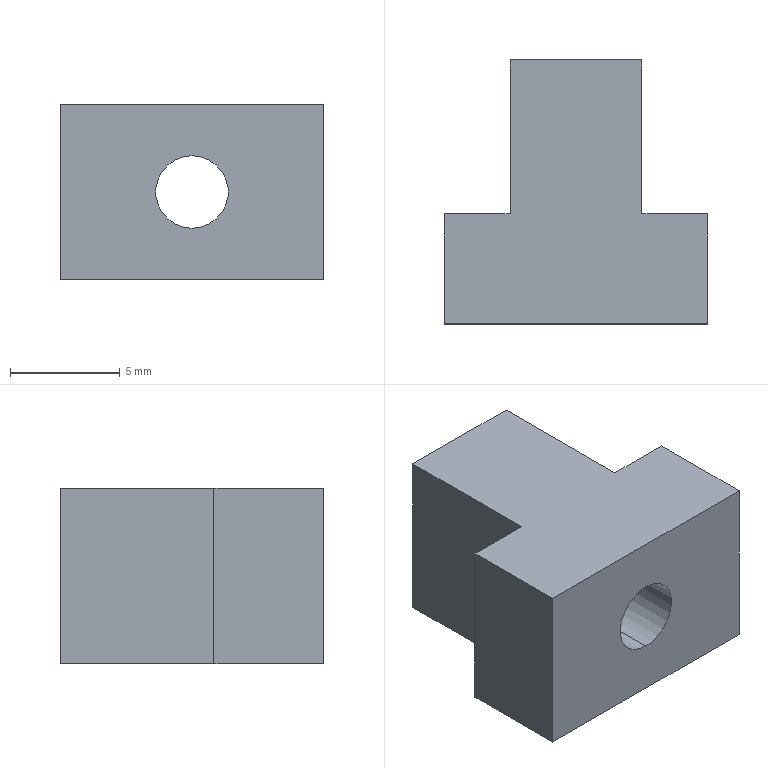Part | STEP file | Shift T-type connector | 1 solid | 12 faces | box 12 x 12 x 8 mm | volume 713.364 mm3 | plane 10 | cylinder 2 | commonest cylinder face diameters 3.3 x2
STEP:
#1=CARTESIAN_POINT('',(0.,0.,0.));
#2=DIRECTION('',(0.,0.,1.));
#3=DIRECTION('',(1.,0.,0.));
#4=AXIS2_PLACEMENT_3D('',#1,#2,#3);
#5=CARTESIAN_POINT('',(6.,0.,5.65));
#6=VERTEX_POINT('',#5);
#7=CARTESIAN_POINT('',(6.,12.,5.65));
#8=VERTEX_POINT('',#7);
#9=CARTESIAN_POINT('',(6.,12.,5.65));
#10=DIRECTION('',(0.,1.,0.));
#11=VECTOR('',#10,1.);
#12=LINE('',#9,#11);
#13=CARTESIAN_POINT('',(6.,12.,4.));
#14=DIRECTION('',(0.,1.,0.));
#15=DIRECTION('',(0.,0.,1.));
#16=AXIS2_PLACEMENT_3D('',#13,#14,#15);
#17=CYLINDRICAL_SURFACE('',#16,1.65);
#18=CARTESIAN_POINT('',(6.283,0.));
#19=DIRECTION('',(0.,1.));
#20=VECTOR('',#19,1.);
#21=LINE('',#18,#20);
#22=(GEOMETRIC_REPRESENTATION_CONTEXT(2)PARAMETRIC_REPRESENTATION_CONTEXT()REPRESENTATION_CONTEXT('',''));
#23=DEFINITIONAL_REPRESENTATION('',(#21),#22);
#24=PCURVE('',#17,#23);
#25=CARTESIAN_POINT('',(6.,12.,4.));
#26=DIRECTION('',(0.,1.,0.));
#27=DIRECTION('',(0.,0.,1.));
#28=AXIS2_PLACEMENT_3D('',#25,#26,#27);
#29=CYLINDRICAL_SURFACE('',#28,1.65);
#30=CARTESIAN_POINT('',(0.,0.));
#31=DIRECTION('',(0.,1.));
#32=VECTOR('',#31,1.);
#33=LINE('',#30,#32);
#34=(GEOMETRIC_REPRESENTATION_CONTEXT(2)PARAMETRIC_REPRESENTATION_CONTEXT()REPRESENTATION_CONTEXT('',''));
#35=DEFINITIONAL_REPRESENTATION('',(#33),#34);
#36=PCURVE('',#29,#35);
#37=SURFACE_CURVE('',#12,(#24,#36),.PCURVE_S1.);
#38=EDGE_CURVE('',#6,#8,#37,.T.);
#39=ORIENTED_EDGE('',*,*,#38,.T.);
#40=CARTESIAN_POINT('',(6.,12.,2.35));
#41=VERTEX_POINT('',#40);
#42=CARTESIAN_POINT('',(6.,12.,4.));
#43=DIRECTION('',(0.,1.,0.));
#44=DIRECTION('',(0.,0.,1.));
#45=AXIS2_PLACEMENT_3D('',#42,#43,#44);
#46=CIRCLE('',#45,1.65);
#47=CARTESIAN_POINT('',(0.,0.));
#48=DIRECTION('',(1.,0.));
#49=VECTOR('',#48,1.);
#50=LINE('',#47,#49);
#51=(GEOMETRIC_REPRESENTATION_CONTEXT(2)PARAMETRIC_REPRESENTATION_CONTEXT()REPRESENTATION_CONTEXT('',''));
#52=DEFINITIONAL_REPRESENTATION('',(#50),#51);
#53=PCURVE('',#17,#52);
#54=CARTESIAN_POINT('',(0.,12.,8.));
#55=DIRECTION('',(0.,-1.,0.));
#56=DIRECTION('',(0.,0.,-1.));
#57=AXIS2_PLACEMENT_3D('',#54,#55,#56);
#58=PLANE('',#57);
#59=CARTESIAN_POINT('',(2.35,6.));
#60=CARTESIAN_POINT('',(2.35,8.858));
#61=CARTESIAN_POINT('',(4.825,7.429));
#62=CARTESIAN_POINT('',(7.3,6.));
#63=CARTESIAN_POINT('',(4.825,4.571));
#64=CARTESIAN_POINT('',(2.35,3.142));
#65=CARTESIAN_POINT('',(2.35,6.));
#66=(BOUNDED_CURVE()B_SPLINE_CURVE(2,(#59,#60,#61,#62,#63,#64,#65),.UNSPECIFIED.,.T.,.F.)B_SPLINE_CURVE_WITH_KNOTS((1,2,2,2,2,1),(-2.094,0.,2.094,4.189,6.283,8.378),.UNSPECIFIED.)CURVE()GEOMETRIC_REPRESENTATION_ITEM()RATIONAL_B_SPLINE_CURVE((1.,0.5,1.,0.5,1.,0.5,1.))REPRESENTATION_ITEM(''));
#67=(GEOMETRIC_REPRESENTATION_CONTEXT(2)PARAMETRIC_REPRESENTATION_CONTEXT()REPRESENTATION_CONTEXT('',''));
#68=DEFINITIONAL_REPRESENTATION('',(#66),#67);
#69=PCURVE('',#58,#68);
#70=SURFACE_CURVE('',#46,(#53,#69),.PCURVE_S1.);
#71=EDGE_CURVE('',#41,#8,#70,.T.);
#72=ORIENTED_EDGE('',*,*,#71,.F.);
#73=CARTESIAN_POINT('',(6.,0.,2.35));
#74=VERTEX_POINT('',#73);
#75=CARTESIAN_POINT('',(6.,12.,2.35));
#76=DIRECTION('',(0.,1.,0.));
#77=VECTOR('',#76,1.);
#78=LINE('',#75,#77);
#79=CARTESIAN_POINT('',(3.142,0.));
#80=DIRECTION('',(0.,1.));
#81=VECTOR('',#80,1.);
#82=LINE('',#79,#81);
#83=(GEOMETRIC_REPRESENTATION_CONTEXT(2)PARAMETRIC_REPRESENTATION_CONTEXT()REPRESENTATION_CONTEXT('',''));
#84=DEFINITIONAL_REPRESENTATION('',(#82),#83);
#85=PCURVE('',#17,#84);
#86=CARTESIAN_POINT('',(3.142,0.));
#87=DIRECTION('',(0.,1.));
#88=VECTOR('',#87,1.);
#89=LINE('',#86,#88);
#90=(GEOMETRIC_REPRESENTATION_CONTEXT(2)PARAMETRIC_REPRESENTATION_CONTEXT()REPRESENTATION_CONTEXT('',''));
#91=DEFINITIONAL_REPRESENTATION('',(#89),#90);
#92=PCURVE('',#29,#91);
#93=SURFACE_CURVE('',#78,(#85,#92),.PCURVE_S1.);
#94=EDGE_CURVE('',#74,#41,#93,.T.);
#95=ORIENTED_EDGE('',*,*,#94,.F.);
#96=CARTESIAN_POINT('',(6.,0.,4.));
#97=DIRECTION('',(0.,1.,0.));
#98=DIRECTION('',(0.,0.,1.));
#99=AXIS2_PLACEMENT_3D('',#96,#97,#98);
#100=CIRCLE('',#99,1.65);
#101=CARTESIAN_POINT('',(0.,-12.));
#102=DIRECTION('',(1.,0.));
#103=VECTOR('',#102,1.);
#104=LINE('',#101,#103);
#105=(GEOMETRIC_REPRESENTATION_CONTEXT(2)PARAMETRIC_REPRESENTATION_CONTEXT()REPRESENTATION_CONTEXT('',''));
#106=DEFINITIONAL_REPRESENTATION('',(#104),#105);
#107=PCURVE('',#17,#106);
#108=CARTESIAN_POINT('',(0.,0.,8.));
#109=DIRECTION('',(0.,1.,0.));
#110=DIRECTION('',(0.,0.,1.));
#111=AXIS2_PLACEMENT_3D('',#108,#109,#110);
#112=PLANE('',#111);
#113=CARTESIAN_POINT('',(-4.,6.));
#114=DIRECTION('',(1.,0.));
#115=AXIS2_PLACEMENT_2D('',#113,#114);
#116=CIRCLE('',#115,1.65);
#117=(GEOMETRIC_REPRESENTATION_CONTEXT(2)PARAMETRIC_REPRESENTATION_CONTEXT()REPRESENTATION_CONTEXT('',''));
#118=DEFINITIONAL_REPRESENTATION('',(#116),#117);
#119=PCURVE('',#112,#118);
#120=SURFACE_CURVE('',#100,(#107,#119),.PCURVE_S1.);
#121=EDGE_CURVE('',#74,#6,#120,.T.);
#122=ORIENTED_EDGE('',*,*,#121,.T.);
#123=EDGE_LOOP('',(#39,#72,#95,#122));
#124=FACE_BOUND('',#123,.F.);
#125=ADVANCED_FACE('',(#124),#17,.F.);
#126=CARTESIAN_POINT('',(0.,5.,8.));
#127=VERTEX_POINT('',#126);
#128=CARTESIAN_POINT('',(0.,0.,8.));
#129=VERTEX_POINT('',#128);
#130=CARTESIAN_POINT('',(0.,0.,8.));
#131=DIRECTION('',(0.,-1.,0.));
#132=VECTOR('',#131,1.);
#133=LINE('',#130,#132);
#134=CARTESIAN_POINT('',(0.,0.,8.));
#135=DIRECTION('',(1.,0.,0.));
#136=DIRECTION('',(0.,0.,-1.));
#137=AXIS2_PLACEMENT_3D('',#134,#135,#136);
#138=PLANE('',#137);
#139=CARTESIAN_POINT('',(0.,0.));
#140=DIRECTION('',(0.,-1.));
#141=VECTOR('',#140,1.);
#142=LINE('',#139,#141);
#143=(GEOMETRIC_REPRESENTATION_CONTEXT(2)PARAMETRIC_REPRESENTATION_CONTEXT()REPRESENTATION_CONTEXT('',''));
#144=DEFINITIONAL_REPRESENTATION('',(#142),#143);
#145=PCURVE('',#138,#144);
#146=CARTESIAN_POINT('',(0.,12.,8.));
#147=DIRECTION('',(0.,0.,-1.));
#148=DIRECTION('',(-1.,0.,0.));
#149=AXIS2_PLACEMENT_3D('',#146,#147,#148);
#150=PLANE('',#149);
#151=CARTESIAN_POINT('',(0.,-12.));
#152=DIRECTION('',(0.,-1.));
#153=VECTOR('',#152,1.);
#154=LINE('',#151,#153);
#155=(GEOMETRIC_REPRESENTATION_CONTEXT(2)PARAMETRIC_REPRESENTATION_CONTEXT()REPRESENTATION_CONTEXT('',''));
#156=DEFINITIONAL_REPRESENTATION('',(#154),#155);
#157=PCURVE('',#150,#156);
#158=SURFACE_CURVE('',#133,(#145,#157),.PCURVE_S1.);
#159=EDGE_CURVE('',#127,#129,#158,.T.);
#160=ORIENTED_EDGE('',*,*,#159,.F.);
#161=CARTESIAN_POINT('',(0.,5.,0.));
#162=VERTEX_POINT('',#161);
#163=CARTESIAN_POINT('',(0.,5.,8.));
#164=DIRECTION('',(0.,0.,-1.));
#165=VECTOR('',#164,1.);
#166=LINE('',#163,#165);
#167=CARTESIAN_POINT('',(0.,5.));
#168=DIRECTION('',(1.,0.));
#169=VECTOR('',#168,1.);
#170=LINE('',#167,#169);
#171=(GEOMETRIC_REPRESENTATION_CONTEXT(2)PARAMETRIC_REPRESENTATION_CONTEXT()REPRESENTATION_CONTEXT('',''));
#172=DEFINITIONAL_REPRESENTATION('',(#170),#171);
#173=PCURVE('',#138,#172);
#174=CARTESIAN_POINT('',(3.,5.,0.));
#175=DIRECTION('',(0.,-1.,0.));
#176=DIRECTION('',(1.,0.,0.));
#177=AXIS2_PLACEMENT_3D('',#174,#175,#176);
#178=PLANE('',#177);
#179=CARTESIAN_POINT('',(-3.,8.));
#180=DIRECTION('',(0.,-1.));
#181=VECTOR('',#180,1.);
#182=LINE('',#179,#181);
#183=(GEOMETRIC_REPRESENTATION_CONTEXT(2)PARAMETRIC_REPRESENTATION_CONTEXT()REPRESENTATION_CONTEXT('',''));
#184=DEFINITIONAL_REPRESENTATION('',(#182),#183);
#185=PCURVE('',#178,#184);
#186=SURFACE_CURVE('',#166,(#173,#185),.PCURVE_S1.);
#187=EDGE_CURVE('',#127,#162,#186,.T.);
#188=ORIENTED_EDGE('',*,*,#187,.T.);
#189=CARTESIAN_POINT('',(0.,0.,0.));
#190=VERTEX_POINT('',#189);
#191=CARTESIAN_POINT('',(0.,0.,0.));
#192=DIRECTION('',(0.,-1.,0.));
#193=VECTOR('',#192,1.);
#194=LINE('',#191,#193);
#195=CARTESIAN_POINT('',(8.,0.));
#196=DIRECTION('',(0.,-1.));
#197=VECTOR('',#196,1.);
#198=LINE('',#195,#197);
#199=(GEOMETRIC_REPRESENTATION_CONTEXT(2)PARAMETRIC_REPRESENTATION_CONTEXT()REPRESENTATION_CONTEXT('',''));
#200=DEFINITIONAL_REPRESENTATION('',(#198),#199);
#201=PCURVE('',#138,#200);
#202=CARTESIAN_POINT('',(0.,12.,0.));
#203=DIRECTION('',(0.,0.,-1.));
#204=DIRECTION('',(-1.,0.,0.));
#205=AXIS2_PLACEMENT_3D('',#202,#203,#204);
#206=PLANE('',#205);
#207=CARTESIAN_POINT('',(0.,-12.));
#208=DIRECTION('',(0.,-1.));
#209=VECTOR('',#208,1.);
#210=LINE('',#207,#209);
#211=(GEOMETRIC_REPRESENTATION_CONTEXT(2)PARAMETRIC_REPRESENTATION_CONTEXT()REPRESENTATION_CONTEXT('',''));
#212=DEFINITIONAL_REPRESENTATION('',(#210),#211);
#213=PCURVE('',#206,#212);
#214=SURFACE_CURVE('',#194,(#201,#213),.PCURVE_S1.);
#215=EDGE_CURVE('',#162,#190,#214,.T.);
#216=ORIENTED_EDGE('',*,*,#215,.T.);
#217=CARTESIAN_POINT('',(0.,0.,8.));
#218=DIRECTION('',(0.,0.,-1.));
#219=VECTOR('',#218,1.);
#220=LINE('',#217,#219);
#221=CARTESIAN_POINT('',(0.,0.));
#222=DIRECTION('',(1.,0.));
#223=VECTOR('',#222,1.);
#224=LINE('',#221,#223);
#225=(GEOMETRIC_REPRESENTATION_CONTEXT(2)PARAMETRIC_REPRESENTATION_CONTEXT()REPRESENTATION_CONTEXT('',''));
#226=DEFINITIONAL_REPRESENTATION('',(#224),#225);
#227=PCURVE('',#138,#226);
#228=CARTESIAN_POINT('',(0.,0.));
#229=DIRECTION('',(-1.,0.));
#230=VECTOR('',#229,1.);
#231=LINE('',#228,#230);
#232=(GEOMETRIC_REPRESENTATION_CONTEXT(2)PARAMETRIC_REPRESENTATION_CONTEXT()REPRESENTATION_CONTEXT('',''));
#233=DEFINITIONAL_REPRESENTATION('',(#231),#232);
#234=PCURVE('',#112,#233);
#235=SURFACE_CURVE('',#220,(#227,#234),.PCURVE_S1.);
#236=EDGE_CURVE('',#129,#190,#235,.T.);
#237=ORIENTED_EDGE('',*,*,#236,.F.);
#238=EDGE_LOOP('',(#160,#188,#216,#237));
#239=FACE_BOUND('',#238,.T.);
#240=ADVANCED_FACE('',(#239),#138,.F.);
#241=CARTESIAN_POINT('',(6.,0.,4.));
#242=DIRECTION('',(0.,1.,0.));
#243=DIRECTION('',(0.,0.,1.));
#244=AXIS2_PLACEMENT_3D('',#241,#242,#243);
#245=CIRCLE('',#244,1.65);
#246=CARTESIAN_POINT('',(-4.,6.));
#247=DIRECTION('',(1.,0.));
#248=AXIS2_PLACEMENT_2D('',#246,#247);
#249=CIRCLE('',#248,1.65);
#250=(GEOMETRIC_REPRESENTATION_CONTEXT(2)PARAMETRIC_REPRESENTATION_CONTEXT()REPRESENTATION_CONTEXT('',''));
#251=DEFINITIONAL_REPRESENTATION('',(#249),#250);
#252=PCURVE('',#112,#251);
#253=CARTESIAN_POINT('',(0.,-12.));
#254=DIRECTION('',(1.,0.));
#255=VECTOR('',#254,1.);
#256=LINE('',#253,#255);
#257=(GEOMETRIC_REPRESENTATION_CONTEXT(2)PARAMETRIC_REPRESENTATION_CONTEXT()REPRESENTATION_CONTEXT('',''));
#258=DEFINITIONAL_REPRESENTATION('',(#256),#257);
#259=PCURVE('',#29,#258);
#260=SURFACE_CURVE('',#245,(#252,#259),.PCURVE_S1.);
#261=EDGE_CURVE('',#6,#74,#260,.T.);
#262=ORIENTED_EDGE('',*,*,#261,.T.);
#263=ORIENTED_EDGE('',*,*,#121,.T.);
#264=EDGE_LOOP('',(#262,#263));
#265=FACE_BOUND('',#264,.T.);
#266=CARTESIAN_POINT('',(12.,0.,0.));
#267=VERTEX_POINT('',#266);
#268=CARTESIAN_POINT('',(0.,0.,0.));
#269=DIRECTION('',(1.,0.,0.));
#270=VECTOR('',#269,1.);
#271=LINE('',#268,#270);
#272=CARTESIAN_POINT('',(-8.,0.));
#273=DIRECTION('',(0.,1.));
#274=VECTOR('',#273,1.);
#275=LINE('',#272,#274);
#276=(GEOMETRIC_REPRESENTATION_CONTEXT(2)PARAMETRIC_REPRESENTATION_CONTEXT()REPRESENTATION_CONTEXT('',''));
#277=DEFINITIONAL_REPRESENTATION('',(#275),#276);
#278=PCURVE('',#112,#277);
#279=CARTESIAN_POINT('',(0.,-12.));
#280=DIRECTION('',(-1.,0.));
#281=VECTOR('',#280,1.);
#282=LINE('',#279,#281);
#283=(GEOMETRIC_REPRESENTATION_CONTEXT(2)PARAMETRIC_REPRESENTATION_CONTEXT()REPRESENTATION_CONTEXT('',''));
#284=DEFINITIONAL_REPRESENTATION('',(#282),#283);
#285=PCURVE('',#206,#284);
#286=SURFACE_CURVE('',#271,(#278,#285),.PCURVE_S1.);
#287=EDGE_CURVE('',#190,#267,#286,.T.);
#288=ORIENTED_EDGE('',*,*,#287,.T.);
#289=CARTESIAN_POINT('',(12.,0.,8.));
#290=VERTEX_POINT('',#289);
#291=CARTESIAN_POINT('',(12.,0.,8.));
#292=DIRECTION('',(0.,0.,-1.));
#293=VECTOR('',#292,1.);
#294=LINE('',#291,#293);
#295=CARTESIAN_POINT('',(0.,12.));
#296=DIRECTION('',(-1.,0.));
#297=VECTOR('',#296,1.);
#298=LINE('',#295,#297);
#299=(GEOMETRIC_REPRESENTATION_CONTEXT(2)PARAMETRIC_REPRESENTATION_CONTEXT()REPRESENTATION_CONTEXT('',''));
#300=DEFINITIONAL_REPRESENTATION('',(#298),#299);
#301=PCURVE('',#112,#300);
#302=CARTESIAN_POINT('',(12.,0.,8.));
#303=DIRECTION('',(-1.,0.,0.));
#304=DIRECTION('',(0.,0.,1.));
#305=AXIS2_PLACEMENT_3D('',#302,#303,#304);
#306=PLANE('',#305);
#307=CARTESIAN_POINT('',(0.,0.));
#308=DIRECTION('',(-1.,0.));
#309=VECTOR('',#308,1.);
#310=LINE('',#307,#309);
#311=(GEOMETRIC_REPRESENTATION_CONTEXT(2)PARAMETRIC_REPRESENTATION_CONTEXT()REPRESENTATION_CONTEXT('',''));
#312=DEFINITIONAL_REPRESENTATION('',(#310),#311);
#313=PCURVE('',#306,#312);
#314=SURFACE_CURVE('',#294,(#301,#313),.PCURVE_S1.);
#315=EDGE_CURVE('',#290,#267,#314,.T.);
#316=ORIENTED_EDGE('',*,*,#315,.F.);
#317=CARTESIAN_POINT('',(0.,0.,8.));
#318=DIRECTION('',(1.,0.,0.));
#319=VECTOR('',#318,1.);
#320=LINE('',#317,#319);
#321=CARTESIAN_POINT('',(0.,0.));
#322=DIRECTION('',(0.,1.));
#323=VECTOR('',#322,1.);
#324=LINE('',#321,#323);
#325=(GEOMETRIC_REPRESENTATION_CONTEXT(2)PARAMETRIC_REPRESENTATION_CONTEXT()REPRESENTATION_CONTEXT('',''));
#326=DEFINITIONAL_REPRESENTATION('',(#324),#325);
#327=PCURVE('',#112,#326);
#328=CARTESIAN_POINT('',(0.,-12.));
#329=DIRECTION('',(-1.,0.));
#330=VECTOR('',#329,1.);
#331=LINE('',#328,#330);
#332=(GEOMETRIC_REPRESENTATION_CONTEXT(2)PARAMETRIC_REPRESENTATION_CONTEXT()REPRESENTATION_CONTEXT('',''));
#333=DEFINITIONAL_REPRESENTATION('',(#331),#332);
#334=PCURVE('',#150,#333);
#335=SURFACE_CURVE('',#320,(#327,#334),.PCURVE_S1.);
#336=EDGE_CURVE('',#129,#290,#335,.T.);
#337=ORIENTED_EDGE('',*,*,#336,.F.);
#338=ORIENTED_EDGE('',*,*,#236,.T.);
#339=EDGE_LOOP('',(#288,#316,#337,#338));
#340=FACE_BOUND('',#339,.T.);
#341=ADVANCED_FACE('',(#265,#340),#112,.F.);
#342=CARTESIAN_POINT('',(12.,5.,0.));
#343=VERTEX_POINT('',#342);
#344=CARTESIAN_POINT('',(12.,0.,0.));
#345=DIRECTION('',(0.,1.,0.));
#346=VECTOR('',#345,1.);
#347=LINE('',#344,#346);
#348=CARTESIAN_POINT('',(-8.,0.));
#349=DIRECTION('',(0.,1.));
#350=VECTOR('',#349,1.);
#351=LINE('',#348,#350);
#352=(GEOMETRIC_REPRESENTATION_CONTEXT(2)PARAMETRIC_REPRESENTATION_CONTEXT()REPRESENTATION_CONTEXT('',''));
#353=DEFINITIONAL_REPRESENTATION('',(#351),#352);
#354=PCURVE('',#306,#353);
#355=CARTESIAN_POINT('',(-12.,-12.));
#356=DIRECTION('',(0.,1.));
#357=VECTOR('',#356,1.);
#358=LINE('',#355,#357);
#359=(GEOMETRIC_REPRESENTATION_CONTEXT(2)PARAMETRIC_REPRESENTATION_CONTEXT()REPRESENTATION_CONTEXT('',''));
#360=DEFINITIONAL_REPRESENTATION('',(#358),#359);
#361=PCURVE('',#206,#360);
#362=SURFACE_CURVE('',#347,(#354,#361),.PCURVE_S1.);
#363=EDGE_CURVE('',#267,#343,#362,.T.);
#364=ORIENTED_EDGE('',*,*,#363,.T.);
#365=CARTESIAN_POINT('',(12.,5.,8.));
#366=VERTEX_POINT('',#365);
#367=CARTESIAN_POINT('',(12.,5.,8.));
#368=DIRECTION('',(0.,0.,1.));
#369=VECTOR('',#368,1.);
#370=LINE('',#367,#369);
#371=CARTESIAN_POINT('',(0.,5.));
#372=DIRECTION('',(1.,0.));
#373=VECTOR('',#372,1.);
#374=LINE('',#371,#373);
#375=(GEOMETRIC_REPRESENTATION_CONTEXT(2)PARAMETRIC_REPRESENTATION_CONTEXT()REPRESENTATION_CONTEXT('',''));
#376=DEFINITIONAL_REPRESENTATION('',(#374),#375);
#377=PCURVE('',#306,#376);
#378=CARTESIAN_POINT('',(13.974,5.,0.));
#379=DIRECTION('',(0.,-1.,0.));
#380=DIRECTION('',(1.,0.,0.));
#381=AXIS2_PLACEMENT_3D('',#378,#379,#380);
#382=PLANE('',#381);
#383=CARTESIAN_POINT('',(-1.974,8.));
#384=DIRECTION('',(0.,1.));
#385=VECTOR('',#384,1.);
#386=LINE('',#383,#385);
#387=(GEOMETRIC_REPRESENTATION_CONTEXT(2)PARAMETRIC_REPRESENTATION_CONTEXT()REPRESENTATION_CONTEXT('',''));
#388=DEFINITIONAL_REPRESENTATION('',(#386),#387);
#389=PCURVE('',#382,#388);
#390=SURFACE_CURVE('',#370,(#377,#389),.PCURVE_S1.);
#391=EDGE_CURVE('',#343,#366,#390,.T.);
#392=ORIENTED_EDGE('',*,*,#391,.T.);
#393=CARTESIAN_POINT('',(12.,0.,8.));
#394=DIRECTION('',(0.,1.,0.));
#395=VECTOR('',#394,1.);
#396=LINE('',#393,#395);
#397=CARTESIAN_POINT('',(0.,0.));
#398=DIRECTION('',(0.,1.));
#399=VECTOR('',#398,1.);
#400=LINE('',#397,#399);
#401=(GEOMETRIC_REPRESENTATION_CONTEXT(2)PARAMETRIC_REPRESENTATION_CONTEXT()REPRESENTATION_CONTEXT('',''));
#402=DEFINITIONAL_REPRESENTATION('',(#400),#401);
#403=PCURVE('',#306,#402);
#404=CARTESIAN_POINT('',(-12.,-12.));
#405=DIRECTION('',(0.,1.));
#406=VECTOR('',#405,1.);
#407=LINE('',#404,#406);
#408=(GEOMETRIC_REPRESENTATION_CONTEXT(2)PARAMETRIC_REPRESENTATION_CONTEXT()REPRESENTATION_CONTEXT('',''));
#409=DEFINITIONAL_REPRESENTATION('',(#407),#408);
#410=PCURVE('',#150,#409);
#411=SURFACE_CURVE('',#396,(#403,#410),.PCURVE_S1.);
#412=EDGE_CURVE('',#290,#366,#411,.T.);
#413=ORIENTED_EDGE('',*,*,#412,.F.);
#414=ORIENTED_EDGE('',*,*,#315,.T.);
#415=EDGE_LOOP('',(#364,#392,#413,#414));
#416=FACE_BOUND('',#415,.T.);
#417=ADVANCED_FACE('',(#416),#306,.F.);
#418=CARTESIAN_POINT('',(6.,12.,4.));
#419=DIRECTION('',(0.,1.,0.));
#420=DIRECTION('',(0.,0.,1.));
#421=AXIS2_PLACEMENT_3D('',#418,#419,#420);
#422=CIRCLE('',#421,1.65);
#423=CARTESIAN_POINT('',(2.35,6.));
#424=CARTESIAN_POINT('',(2.35,8.858));
#425=CARTESIAN_POINT('',(4.825,7.429));
#426=CARTESIAN_POINT('',(7.3,6.));
#427=CARTESIAN_POINT('',(4.825,4.571));
#428=CARTESIAN_POINT('',(2.35,3.142));
#429=CARTESIAN_POINT('',(2.35,6.));
#430=(BOUNDED_CURVE()B_SPLINE_CURVE(2,(#423,#424,#425,#426,#427,#428,#429),.UNSPECIFIED.,.T.,.F.)B_SPLINE_CURVE_WITH_KNOTS((1,2,2,2,2,1),(-2.094,0.,2.094,4.189,6.283,8.378),.UNSPECIFIED.)CURVE()GEOMETRIC_REPRESENTATION_ITEM()RATIONAL_B_SPLINE_CURVE((1.,0.5,1.,0.5,1.,0.5,1.))REPRESENTATION_ITEM(''));
#431=(GEOMETRIC_REPRESENTATION_CONTEXT(2)PARAMETRIC_REPRESENTATION_CONTEXT()REPRESENTATION_CONTEXT('',''));
#432=DEFINITIONAL_REPRESENTATION('',(#430),#431);
#433=PCURVE('',#58,#432);
#434=CARTESIAN_POINT('',(0.,0.));
#435=DIRECTION('',(1.,0.));
#436=VECTOR('',#435,1.);
#437=LINE('',#434,#436);
#438=(GEOMETRIC_REPRESENTATION_CONTEXT(2)PARAMETRIC_REPRESENTATION_CONTEXT()REPRESENTATION_CONTEXT('',''));
#439=DEFINITIONAL_REPRESENTATION('',(#437),#438);
#440=PCURVE('',#29,#439);
#441=SURFACE_CURVE('',#422,(#433,#440),.PCURVE_S1.);
#442=EDGE_CURVE('',#8,#41,#441,.T.);
#443=ORIENTED_EDGE('',*,*,#442,.F.);
#444=ORIENTED_EDGE('',*,*,#71,.F.);
#445=EDGE_LOOP('',(#443,#444));
#446=FACE_BOUND('',#445,.T.);
#447=CARTESIAN_POINT('',(9.,12.,0.));
#448=VERTEX_POINT('',#447);
#449=CARTESIAN_POINT('',(3.,12.,0.));
#450=VERTEX_POINT('',#449);
#451=CARTESIAN_POINT('',(0.,12.,0.));
#452=DIRECTION('',(-1.,0.,0.));
#453=VECTOR('',#452,1.);
#454=LINE('',#451,#453);
#455=CARTESIAN_POINT('',(8.,0.));
#456=DIRECTION('',(0.,-1.));
#457=VECTOR('',#456,1.);
#458=LINE('',#455,#457);
#459=(GEOMETRIC_REPRESENTATION_CONTEXT(2)PARAMETRIC_REPRESENTATION_CONTEXT()REPRESENTATION_CONTEXT('',''));
#460=DEFINITIONAL_REPRESENTATION('',(#458),#459);
#461=PCURVE('',#58,#460);
#462=CARTESIAN_POINT('',(0.,0.));
#463=DIRECTION('',(1.,0.));
#464=VECTOR('',#463,1.);
#465=LINE('',#462,#464);
#466=(GEOMETRIC_REPRESENTATION_CONTEXT(2)PARAMETRIC_REPRESENTATION_CONTEXT()REPRESENTATION_CONTEXT('',''));
#467=DEFINITIONAL_REPRESENTATION('',(#465),#466);
#468=PCURVE('',#206,#467);
#469=SURFACE_CURVE('',#454,(#461,#468),.PCURVE_S1.);
#470=EDGE_CURVE('',#448,#450,#469,.T.);
#471=ORIENTED_EDGE('',*,*,#470,.T.);
#472=CARTESIAN_POINT('',(3.,12.,8.));
#473=VERTEX_POINT('',#472);
#474=CARTESIAN_POINT('',(3.,12.,8.));
#475=DIRECTION('',(0.,0.,1.));
#476=VECTOR('',#475,1.);
#477=LINE('',#474,#476);
#478=CARTESIAN_POINT('',(0.,3.));
#479=DIRECTION('',(-1.,0.));
#480=VECTOR('',#479,1.);
#481=LINE('',#478,#480);
#482=(GEOMETRIC_REPRESENTATION_CONTEXT(2)PARAMETRIC_REPRESENTATION_CONTEXT()REPRESENTATION_CONTEXT('',''));
#483=DEFINITIONAL_REPRESENTATION('',(#481),#482);
#484=PCURVE('',#58,#483);
#485=CARTESIAN_POINT('',(3.,18.435,0.));
#486=DIRECTION('',(1.,0.,0.));
#487=DIRECTION('',(0.,1.,0.));
#488=AXIS2_PLACEMENT_3D('',#485,#486,#487);
#489=PLANE('',#488);
#490=CARTESIAN_POINT('',(-6.435,8.));
#491=DIRECTION('',(0.,1.));
#492=VECTOR('',#491,1.);
#493=LINE('',#490,#492);
#494=(GEOMETRIC_REPRESENTATION_CONTEXT(2)PARAMETRIC_REPRESENTATION_CONTEXT()REPRESENTATION_CONTEXT('',''));
#495=DEFINITIONAL_REPRESENTATION('',(#493),#494);
#496=PCURVE('',#489,#495);
#497=SURFACE_CURVE('',#477,(#484,#496),.PCURVE_S1.);
#498=EDGE_CURVE('',#450,#473,#497,.T.);
#499=ORIENTED_EDGE('',*,*,#498,.T.);
#500=CARTESIAN_POINT('',(9.,12.,8.));
#501=VERTEX_POINT('',#500);
#502=CARTESIAN_POINT('',(0.,12.,8.));
#503=DIRECTION('',(-1.,0.,0.));
#504=VECTOR('',#503,1.);
#505=LINE('',#502,#504);
#506=CARTESIAN_POINT('',(0.,0.));
#507=DIRECTION('',(0.,-1.));
#508=VECTOR('',#507,1.);
#509=LINE('',#506,#508);
#510=(GEOMETRIC_REPRESENTATION_CONTEXT(2)PARAMETRIC_REPRESENTATION_CONTEXT()REPRESENTATION_CONTEXT('',''));
#511=DEFINITIONAL_REPRESENTATION('',(#509),#510);
#512=PCURVE('',#58,#511);
#513=CARTESIAN_POINT('',(0.,0.));
#514=DIRECTION('',(1.,0.));
#515=VECTOR('',#514,1.);
#516=LINE('',#513,#515);
#517=(GEOMETRIC_REPRESENTATION_CONTEXT(2)PARAMETRIC_REPRESENTATION_CONTEXT()REPRESENTATION_CONTEXT('',''));
#518=DEFINITIONAL_REPRESENTATION('',(#516),#517);
#519=PCURVE('',#150,#518);
#520=SURFACE_CURVE('',#505,(#512,#519),.PCURVE_S1.);
#521=EDGE_CURVE('',#501,#473,#520,.T.);
#522=ORIENTED_EDGE('',*,*,#521,.F.);
#523=CARTESIAN_POINT('',(9.,12.,8.));
#524=DIRECTION('',(0.,0.,-1.));
#525=VECTOR('',#524,1.);
#526=LINE('',#523,#525);
#527=CARTESIAN_POINT('',(0.,9.));
#528=DIRECTION('',(1.,0.));
#529=VECTOR('',#528,1.);
#530=LINE('',#527,#529);
#531=(GEOMETRIC_REPRESENTATION_CONTEXT(2)PARAMETRIC_REPRESENTATION_CONTEXT()REPRESENTATION_CONTEXT('',''));
#532=DEFINITIONAL_REPRESENTATION('',(#530),#531);
#533=PCURVE('',#58,#532);
#534=CARTESIAN_POINT('',(9.,16.359,0.));
#535=DIRECTION('',(-1.,0.,0.));
#536=DIRECTION('',(0.,-1.,0.));
#537=AXIS2_PLACEMENT_3D('',#534,#535,#536);
#538=PLANE('',#537);
#539=CARTESIAN_POINT('',(4.359,8.));
#540=DIRECTION('',(0.,-1.));
#541=VECTOR('',#540,1.);
#542=LINE('',#539,#541);
#543=(GEOMETRIC_REPRESENTATION_CONTEXT(2)PARAMETRIC_REPRESENTATION_CONTEXT()REPRESENTATION_CONTEXT('',''));
#544=DEFINITIONAL_REPRESENTATION('',(#542),#543);
#545=PCURVE('',#538,#544);
#546=SURFACE_CURVE('',#526,(#533,#545),.PCURVE_S1.);
#547=EDGE_CURVE('',#501,#448,#546,.T.);
#548=ORIENTED_EDGE('',*,*,#547,.T.);
#549=EDGE_LOOP('',(#471,#499,#522,#548));
#550=FACE_BOUND('',#549,.T.);
#551=ADVANCED_FACE('',(#446,#550),#58,.F.);
#552=ORIENTED_EDGE('',*,*,#521,.T.);
#553=CARTESIAN_POINT('',(3.,5.,8.));
#554=VERTEX_POINT('',#553);
#555=CARTESIAN_POINT('',(3.,18.435,8.));
#556=DIRECTION('',(0.,1.,0.));
#557=VECTOR('',#556,1.);
#558=LINE('',#555,#557);
#559=CARTESIAN_POINT('',(-3.,6.435));
#560=DIRECTION('',(0.,1.));
#561=VECTOR('',#560,1.);
#562=LINE('',#559,#561);
#563=(GEOMETRIC_REPRESENTATION_CONTEXT(2)PARAMETRIC_REPRESENTATION_CONTEXT()REPRESENTATION_CONTEXT('',''));
#564=DEFINITIONAL_REPRESENTATION('',(#562),#563);
#565=PCURVE('',#150,#564);
#566=CARTESIAN_POINT('',(0.,8.));
#567=DIRECTION('',(1.,0.));
#568=VECTOR('',#567,1.);
#569=LINE('',#566,#568);
#570=(GEOMETRIC_REPRESENTATION_CONTEXT(2)PARAMETRIC_REPRESENTATION_CONTEXT()REPRESENTATION_CONTEXT('',''));
#571=DEFINITIONAL_REPRESENTATION('',(#569),#570);
#572=PCURVE('',#489,#571);
#573=SURFACE_CURVE('',#558,(#565,#572),.PCURVE_S1.);
#574=EDGE_CURVE('',#554,#473,#573,.T.);
#575=ORIENTED_EDGE('',*,*,#574,.F.);
#576=CARTESIAN_POINT('',(3.,5.,8.));
#577=DIRECTION('',(1.,0.,0.));
#578=VECTOR('',#577,1.);
#579=LINE('',#576,#578);
#580=CARTESIAN_POINT('',(-3.,-7.));
#581=DIRECTION('',(-1.,0.));
#582=VECTOR('',#581,1.);
#583=LINE('',#580,#582);
#584=(GEOMETRIC_REPRESENTATION_CONTEXT(2)PARAMETRIC_REPRESENTATION_CONTEXT()REPRESENTATION_CONTEXT('',''));
#585=DEFINITIONAL_REPRESENTATION('',(#583),#584);
#586=PCURVE('',#150,#585);
#587=CARTESIAN_POINT('',(0.,8.));
#588=DIRECTION('',(1.,0.));
#589=VECTOR('',#588,1.);
#590=LINE('',#587,#589);
#591=(GEOMETRIC_REPRESENTATION_CONTEXT(2)PARAMETRIC_REPRESENTATION_CONTEXT()REPRESENTATION_CONTEXT('',''));
#592=DEFINITIONAL_REPRESENTATION('',(#590),#591);
#593=PCURVE('',#178,#592);
#594=SURFACE_CURVE('',#579,(#586,#593),.PCURVE_S1.);
#595=EDGE_CURVE('',#127,#554,#594,.T.);
#596=ORIENTED_EDGE('',*,*,#595,.F.);
#597=ORIENTED_EDGE('',*,*,#159,.T.);
#598=ORIENTED_EDGE('',*,*,#336,.T.);
#599=ORIENTED_EDGE('',*,*,#412,.T.);
#600=CARTESIAN_POINT('',(9.,5.,8.));
#601=VERTEX_POINT('',#600);
#602=CARTESIAN_POINT('',(13.974,5.,8.));
#603=DIRECTION('',(1.,0.,0.));
#604=VECTOR('',#603,1.);
#605=LINE('',#602,#604);
#606=CARTESIAN_POINT('',(-13.974,-7.));
#607=DIRECTION('',(-1.,0.));
#608=VECTOR('',#607,1.);
#609=LINE('',#606,#608);
#610=(GEOMETRIC_REPRESENTATION_CONTEXT(2)PARAMETRIC_REPRESENTATION_CONTEXT()REPRESENTATION_CONTEXT('',''));
#611=DEFINITIONAL_REPRESENTATION('',(#609),#610);
#612=PCURVE('',#150,#611);
#613=CARTESIAN_POINT('',(0.,8.));
#614=DIRECTION('',(1.,0.));
#615=VECTOR('',#614,1.);
#616=LINE('',#613,#615);
#617=(GEOMETRIC_REPRESENTATION_CONTEXT(2)PARAMETRIC_REPRESENTATION_CONTEXT()REPRESENTATION_CONTEXT('',''));
#618=DEFINITIONAL_REPRESENTATION('',(#616),#617);
#619=PCURVE('',#382,#618);
#620=SURFACE_CURVE('',#605,(#612,#619),.PCURVE_S1.);
#621=EDGE_CURVE('',#601,#366,#620,.T.);
#622=ORIENTED_EDGE('',*,*,#621,.F.);
#623=CARTESIAN_POINT('',(9.,16.359,8.));
#624=DIRECTION('',(0.,-1.,0.));
#625=VECTOR('',#624,1.);
#626=LINE('',#623,#625);
#627=CARTESIAN_POINT('',(-9.,4.359));
#628=DIRECTION('',(0.,-1.));
#629=VECTOR('',#628,1.);
#630=LINE('',#627,#629);
#631=(GEOMETRIC_REPRESENTATION_CONTEXT(2)PARAMETRIC_REPRESENTATION_CONTEXT()REPRESENTATION_CONTEXT('',''));
#632=DEFINITIONAL_REPRESENTATION('',(#630),#631);
#633=PCURVE('',#150,#632);
#634=CARTESIAN_POINT('',(0.,8.));
#635=DIRECTION('',(1.,0.));
#636=VECTOR('',#635,1.);
#637=LINE('',#634,#636);
#638=(GEOMETRIC_REPRESENTATION_CONTEXT(2)PARAMETRIC_REPRESENTATION_CONTEXT()REPRESENTATION_CONTEXT('',''));
#639=DEFINITIONAL_REPRESENTATION('',(#637),#638);
#640=PCURVE('',#538,#639);
#641=SURFACE_CURVE('',#626,(#633,#640),.PCURVE_S1.);
#642=EDGE_CURVE('',#501,#601,#641,.T.);
#643=ORIENTED_EDGE('',*,*,#642,.F.);
#644=EDGE_LOOP('',(#552,#575,#596,#597,#598,#599,#622,#643));
#645=FACE_BOUND('',#644,.T.);
#646=ADVANCED_FACE('',(#645),#150,.F.);
#647=CARTESIAN_POINT('',(3.,5.,0.));
#648=VERTEX_POINT('',#647);
#649=CARTESIAN_POINT('',(3.,18.435,0.));
#650=DIRECTION('',(0.,1.,0.));
#651=VECTOR('',#650,1.);
#652=LINE('',#649,#651);
#653=CARTESIAN_POINT('',(-3.,6.435));
#654=DIRECTION('',(0.,1.));
#655=VECTOR('',#654,1.);
#656=LINE('',#653,#655);
#657=(GEOMETRIC_REPRESENTATION_CONTEXT(2)PARAMETRIC_REPRESENTATION_CONTEXT()REPRESENTATION_CONTEXT('',''));
#658=DEFINITIONAL_REPRESENTATION('',(#656),#657);
#659=PCURVE('',#206,#658);
#660=CARTESIAN_POINT('',(0.,0.));
#661=DIRECTION('',(1.,0.));
#662=VECTOR('',#661,1.);
#663=LINE('',#660,#662);
#664=(GEOMETRIC_REPRESENTATION_CONTEXT(2)PARAMETRIC_REPRESENTATION_CONTEXT()REPRESENTATION_CONTEXT('',''));
#665=DEFINITIONAL_REPRESENTATION('',(#663),#664);
#666=PCURVE('',#489,#665);
#667=SURFACE_CURVE('',#652,(#659,#666),.PCURVE_S1.);
#668=EDGE_CURVE('',#648,#450,#667,.T.);
#669=ORIENTED_EDGE('',*,*,#668,.T.);
#670=ORIENTED_EDGE('',*,*,#470,.F.);
#671=CARTESIAN_POINT('',(9.,5.,0.));
#672=VERTEX_POINT('',#671);
#673=CARTESIAN_POINT('',(9.,12.,0.));
#674=DIRECTION('',(0.,1.,0.));
#675=VECTOR('',#674,1.);
#676=LINE('',#673,#675);
#677=CARTESIAN_POINT('',(-9.,0.));
#678=DIRECTION('',(0.,1.));
#679=VECTOR('',#678,1.);
#680=LINE('',#677,#679);
#681=(GEOMETRIC_REPRESENTATION_CONTEXT(2)PARAMETRIC_REPRESENTATION_CONTEXT()REPRESENTATION_CONTEXT('',''));
#682=DEFINITIONAL_REPRESENTATION('',(#680),#681);
#683=PCURVE('',#206,#682);
#684=CARTESIAN_POINT('',(4.359,0.));
#685=DIRECTION('',(-1.,0.));
#686=VECTOR('',#685,1.);
#687=LINE('',#684,#686);
#688=(GEOMETRIC_REPRESENTATION_CONTEXT(2)PARAMETRIC_REPRESENTATION_CONTEXT()REPRESENTATION_CONTEXT('',''));
#689=DEFINITIONAL_REPRESENTATION('',(#687),#688);
#690=PCURVE('',#538,#689);
#691=SURFACE_CURVE('',#676,(#683,#690),.PCURVE_S1.);
#692=EDGE_CURVE('',#672,#448,#691,.T.);
#693=ORIENTED_EDGE('',*,*,#692,.F.);
#694=CARTESIAN_POINT('',(13.974,5.,0.));
#695=DIRECTION('',(1.,0.,0.));
#696=VECTOR('',#695,1.);
#697=LINE('',#694,#696);
#698=CARTESIAN_POINT('',(-13.974,-7.));
#699=DIRECTION('',(-1.,0.));
#700=VECTOR('',#699,1.);
#701=LINE('',#698,#700);
#702=(GEOMETRIC_REPRESENTATION_CONTEXT(2)PARAMETRIC_REPRESENTATION_CONTEXT()REPRESENTATION_CONTEXT('',''));
#703=DEFINITIONAL_REPRESENTATION('',(#701),#702);
#704=PCURVE('',#206,#703);
#705=CARTESIAN_POINT('',(0.,0.));
#706=DIRECTION('',(1.,0.));
#707=VECTOR('',#706,1.);
#708=LINE('',#705,#707);
#709=(GEOMETRIC_REPRESENTATION_CONTEXT(2)PARAMETRIC_REPRESENTATION_CONTEXT()REPRESENTATION_CONTEXT('',''));
#710=DEFINITIONAL_REPRESENTATION('',(#708),#709);
#711=PCURVE('',#382,#710);
#712=SURFACE_CURVE('',#697,(#704,#711),.PCURVE_S1.);
#713=EDGE_CURVE('',#672,#343,#712,.T.);
#714=ORIENTED_EDGE('',*,*,#713,.T.);
#715=ORIENTED_EDGE('',*,*,#363,.F.);
#716=ORIENTED_EDGE('',*,*,#287,.F.);
#717=ORIENTED_EDGE('',*,*,#215,.F.);
#718=CARTESIAN_POINT('',(0.,5.,0.));
#719=DIRECTION('',(-1.,0.,0.));
#720=VECTOR('',#719,1.);
#721=LINE('',#718,#720);
#722=CARTESIAN_POINT('',(0.,-7.));
#723=DIRECTION('',(1.,0.));
#724=VECTOR('',#723,1.);
#725=LINE('',#722,#724);
#726=(GEOMETRIC_REPRESENTATION_CONTEXT(2)PARAMETRIC_REPRESENTATION_CONTEXT()REPRESENTATION_CONTEXT('',''));
#727=DEFINITIONAL_REPRESENTATION('',(#725),#726);
#728=PCURVE('',#206,#727);
#729=CARTESIAN_POINT('',(-3.,0.));
#730=DIRECTION('',(-1.,0.));
#731=VECTOR('',#730,1.);
#732=LINE('',#729,#731);
#733=(GEOMETRIC_REPRESENTATION_CONTEXT(2)PARAMETRIC_REPRESENTATION_CONTEXT()REPRESENTATION_CONTEXT('',''));
#734=DEFINITIONAL_REPRESENTATION('',(#732),#733);
#735=PCURVE('',#178,#734);
#736=SURFACE_CURVE('',#721,(#728,#735),.PCURVE_S1.);
#737=EDGE_CURVE('',#648,#162,#736,.T.);
#738=ORIENTED_EDGE('',*,*,#737,.F.);
#739=EDGE_LOOP('',(#669,#670,#693,#714,#715,#716,#717,#738));
#740=FACE_BOUND('',#739,.T.);
#741=ADVANCED_FACE('',(#740),#206,.T.);
#742=ORIENTED_EDGE('',*,*,#713,.F.);
#743=CARTESIAN_POINT('',(9.,5.,0.));
#744=DIRECTION('',(0.,0.,1.));
#745=VECTOR('',#744,1.);
#746=LINE('',#743,#745);
#747=CARTESIAN_POINT('',(-4.974,0.));
#748=DIRECTION('',(0.,1.));
#749=VECTOR('',#748,1.);
#750=LINE('',#747,#749);
#751=(GEOMETRIC_REPRESENTATION_CONTEXT(2)PARAMETRIC_REPRESENTATION_CONTEXT()REPRESENTATION_CONTEXT('',''));
#752=DEFINITIONAL_REPRESENTATION('',(#750),#751);
#753=PCURVE('',#382,#752);
#754=CARTESIAN_POINT('',(11.359,0.));
#755=DIRECTION('',(0.,1.));
#756=VECTOR('',#755,1.);
#757=LINE('',#754,#756);
#758=(GEOMETRIC_REPRESENTATION_CONTEXT(2)PARAMETRIC_REPRESENTATION_CONTEXT()REPRESENTATION_CONTEXT('',''));
#759=DEFINITIONAL_REPRESENTATION('',(#757),#758);
#760=PCURVE('',#538,#759);
#761=SURFACE_CURVE('',#746,(#753,#760),.PCURVE_S1.);
#762=EDGE_CURVE('',#672,#601,#761,.T.);
#763=ORIENTED_EDGE('',*,*,#762,.T.);
#764=ORIENTED_EDGE('',*,*,#621,.T.);
#765=ORIENTED_EDGE('',*,*,#391,.F.);
#766=EDGE_LOOP('',(#742,#763,#764,#765));
#767=FACE_BOUND('',#766,.T.);
#768=ADVANCED_FACE('',(#767),#382,.F.);
#769=ORIENTED_EDGE('',*,*,#642,.T.);
#770=ORIENTED_EDGE('',*,*,#762,.F.);
#771=ORIENTED_EDGE('',*,*,#692,.T.);
#772=ORIENTED_EDGE('',*,*,#547,.F.);
#773=EDGE_LOOP('',(#769,#770,#771,#772));
#774=FACE_BOUND('',#773,.T.);
#775=ADVANCED_FACE('',(#774),#538,.F.);
#776=ORIENTED_EDGE('',*,*,#668,.F.);
#777=CARTESIAN_POINT('',(3.,5.,0.));
#778=DIRECTION('',(0.,0.,1.));
#779=VECTOR('',#778,1.);
#780=LINE('',#777,#779);
#781=CARTESIAN_POINT('',(-13.435,0.));
#782=DIRECTION('',(0.,1.));
#783=VECTOR('',#782,1.);
#784=LINE('',#781,#783);
#785=(GEOMETRIC_REPRESENTATION_CONTEXT(2)PARAMETRIC_REPRESENTATION_CONTEXT()REPRESENTATION_CONTEXT('',''));
#786=DEFINITIONAL_REPRESENTATION('',(#784),#785);
#787=PCURVE('',#489,#786);
#788=CARTESIAN_POINT('',(0.,0.));
#789=DIRECTION('',(0.,1.));
#790=VECTOR('',#789,1.);
#791=LINE('',#788,#790);
#792=(GEOMETRIC_REPRESENTATION_CONTEXT(2)PARAMETRIC_REPRESENTATION_CONTEXT()REPRESENTATION_CONTEXT('',''));
#793=DEFINITIONAL_REPRESENTATION('',(#791),#792);
#794=PCURVE('',#178,#793);
#795=SURFACE_CURVE('',#780,(#787,#794),.PCURVE_S1.);
#796=EDGE_CURVE('',#648,#554,#795,.T.);
#797=ORIENTED_EDGE('',*,*,#796,.T.);
#798=ORIENTED_EDGE('',*,*,#574,.T.);
#799=ORIENTED_EDGE('',*,*,#498,.F.);
#800=EDGE_LOOP('',(#776,#797,#798,#799));
#801=FACE_BOUND('',#800,.T.);
#802=ADVANCED_FACE('',(#801),#489,.F.);
#803=ORIENTED_EDGE('',*,*,#595,.T.);
#804=ORIENTED_EDGE('',*,*,#796,.F.);
#805=ORIENTED_EDGE('',*,*,#737,.T.);
#806=ORIENTED_EDGE('',*,*,#187,.F.);
#807=EDGE_LOOP('',(#803,#804,#805,#806));
#808=FACE_BOUND('',#807,.T.);
#809=ADVANCED_FACE('',(#808),#178,.F.);
#810=ORIENTED_EDGE('',*,*,#442,.F.);
#811=ORIENTED_EDGE('',*,*,#38,.F.);
#812=ORIENTED_EDGE('',*,*,#261,.T.);
#813=ORIENTED_EDGE('',*,*,#94,.T.);
#814=EDGE_LOOP('',(#810,#811,#812,#813));
#815=FACE_BOUND('',#814,.F.);
#816=ADVANCED_FACE('',(#815),#29,.F.);
#817=CLOSED_SHELL('',(#125,#240,#341,#417,#551,#646,#741,#768,#775,#802,#809,#816));
#818=MANIFOLD_SOLID_BREP('',#817);
#819=(LENGTH_UNIT()NAMED_UNIT(*)SI_UNIT(.MILLI.,.METRE.));
#820=UNCERTAINTY_MEASURE_WITH_UNIT(LENGTH_MEASURE(0.0000001),#819,'','');
#821=(NAMED_UNIT(*)PLANE_ANGLE_UNIT()SI_UNIT($,.RADIAN.));
#822=(NAMED_UNIT(*)SI_UNIT($,.STERADIAN.)SOLID_ANGLE_UNIT());
#823=(GEOMETRIC_REPRESENTATION_CONTEXT(3)GLOBAL_UNCERTAINTY_ASSIGNED_CONTEXT((#820))GLOBAL_UNIT_ASSIGNED_CONTEXT((#819,#821,#822))REPRESENTATION_CONTEXT('',''));
#824=ADVANCED_BREP_SHAPE_REPRESENTATION('',(#4,#818),#823);